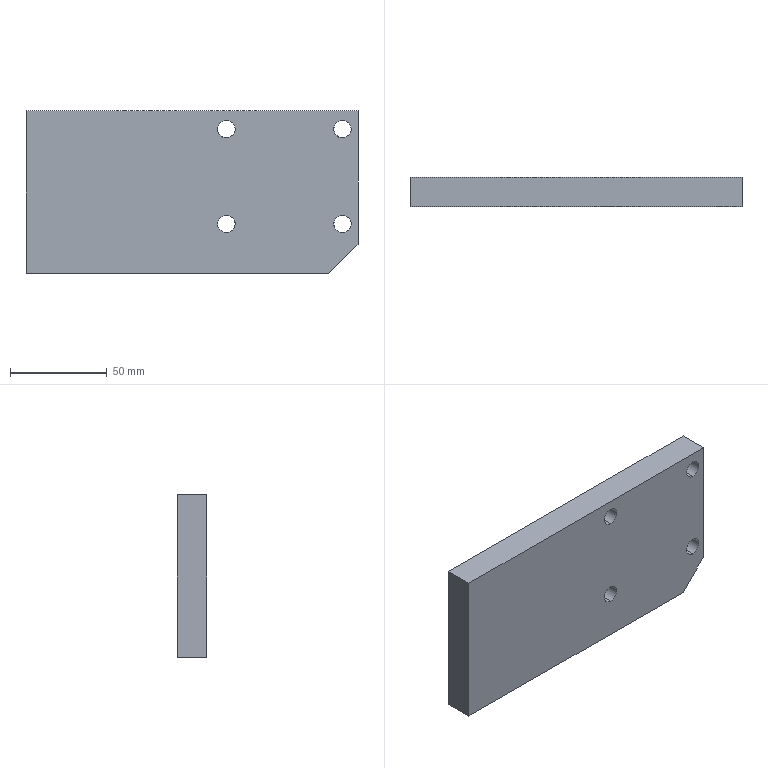Part | STEP file | Positioning_id1690_x_t | 1 solid | 15 faces | box 171.5 x 15 x 84 mm | volume 210585 mm3 | cylinder 8 | plane 7 | commonest cylinder face diameters 9 x8